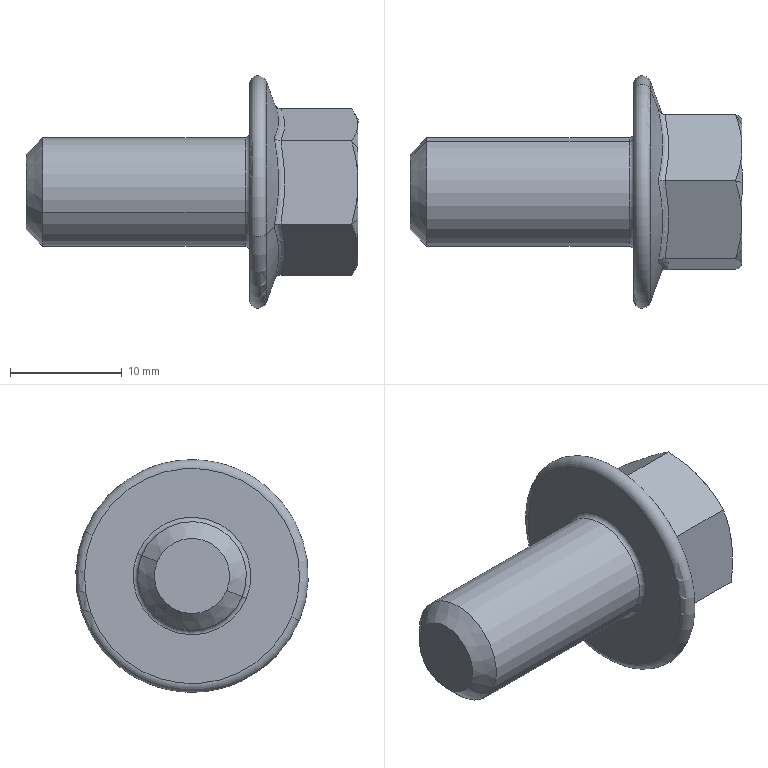Part | SolidWorks | features BaseBody 1 | 1 solid | 40 faces | box 29.7 x 20.8 x 20.8 mm | volume 3100 mm3 | cone 16 | plane 10 | spline 6 | cylinder 4 | torus 4 | commonest cylinder face diameters 9.732 x2 10.4 x2